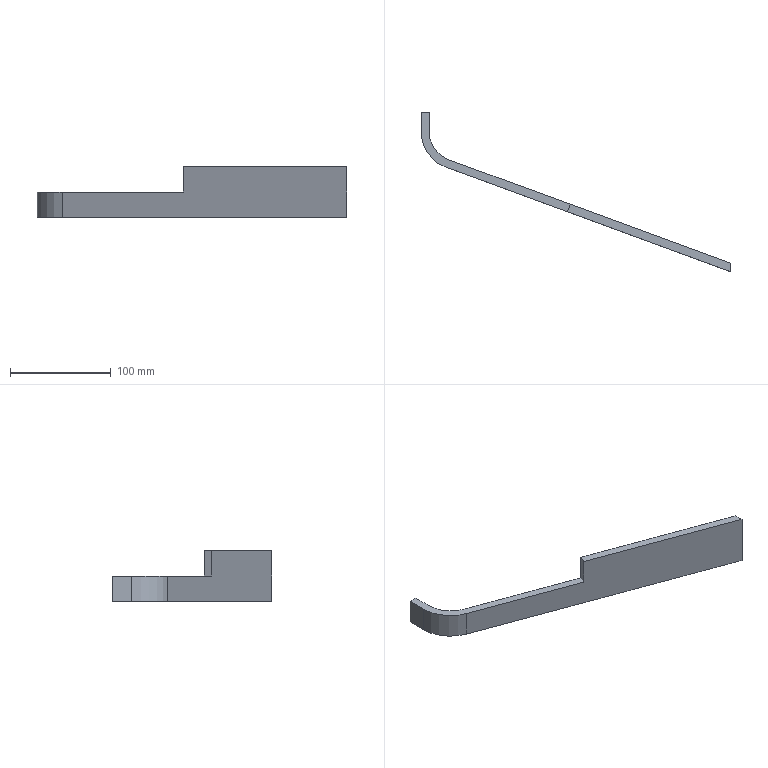Part | SolidWorks | features Extrusion 1, ICE 1 | 1 solid | 12 faces | box 308 x 158.521 x 50 mm | volume 106428 mm3 | plane 10 | cylinder 2 | commonest cylinder face diameters 60 x1 76 x1
STEP:
#1=CARTESIAN_POINT('',(-150.5,75.5,25.));
#2=VERTEX_POINT('',#1);
#3=CARTESIAN_POINT('',(-158.5,75.5,25.));
#4=VERTEX_POINT('',#3);
#5=CARTESIAN_POINT('',(-158.5,75.5,25.));
#6=DIRECTION('',(-1.,0.,0.));
#7=VECTOR('',#6,1000.);
#8=LINE('',#5,#7);
#9=EDGE_CURVE('',#2,#4,#8,.T.);
#10=ORIENTED_EDGE('',*,*,#9,.F.);
#11=CARTESIAN_POINT('',(-150.5,75.5,0.));
#12=VERTEX_POINT('',#11);
#13=CARTESIAN_POINT('',(-150.5,75.5,50.));
#14=DIRECTION('',(0.,0.,-1.));
#15=VECTOR('',#14,1000.);
#16=LINE('',#13,#15);
#17=EDGE_CURVE('',#2,#12,#16,.T.);
#18=ORIENTED_EDGE('',*,*,#17,.T.);
#19=CARTESIAN_POINT('',(-158.5,75.5,0.));
#20=VERTEX_POINT('',#19);
#21=CARTESIAN_POINT('',(-158.5,75.5,0.));
#22=DIRECTION('',(-1.,0.,0.));
#23=VECTOR('',#22,1000.);
#24=LINE('',#21,#23);
#25=EDGE_CURVE('',#12,#20,#24,.T.);
#26=ORIENTED_EDGE('',*,*,#25,.T.);
#27=CARTESIAN_POINT('',(-158.5,75.5,50.));
#28=DIRECTION('',(0.,0.,-1.));
#29=VECTOR('',#28,1000.);
#30=LINE('',#27,#29);
#31=EDGE_CURVE('',#4,#20,#30,.T.);
#32=ORIENTED_EDGE('',*,*,#31,.F.);
#33=EDGE_LOOP('',(#10,#18,#26,#32));
#34=FACE_OUTER_BOUND('',#33,.T.);
#35=CARTESIAN_POINT('',(-158.5,75.5,50.));
#36=DIRECTION('',(0.,-1.,0.));
#37=DIRECTION('',(0.,0.,-1.));
#38=AXIS2_PLACEMENT_3D('',#35,#36,#37);
#39=PLANE('',#38);
#40=ADVANCED_FACE('',(#34),#39,.F.);
#41=CARTESIAN_POINT('',(-158.5,56.453,25.));
#42=VERTEX_POINT('',#41);
#43=CARTESIAN_POINT('',(-158.5,75.5,25.));
#44=DIRECTION('',(0.,-1.,0.));
#45=VECTOR('',#44,1000.);
#46=LINE('',#43,#45);
#47=EDGE_CURVE('',#4,#42,#46,.T.);
#48=ORIENTED_EDGE('',*,*,#47,.F.);
#49=ORIENTED_EDGE('',*,*,#31,.T.);
#50=CARTESIAN_POINT('',(-158.5,56.453,0.));
#51=VERTEX_POINT('',#50);
#52=CARTESIAN_POINT('',(-158.5,75.5,0.));
#53=DIRECTION('',(0.,-1.,0.));
#54=VECTOR('',#53,1000.);
#55=LINE('',#52,#54);
#56=EDGE_CURVE('',#20,#51,#55,.T.);
#57=ORIENTED_EDGE('',*,*,#56,.T.);
#58=CARTESIAN_POINT('',(-158.5,56.453,50.));
#59=DIRECTION('',(0.,0.,-1.));
#60=VECTOR('',#59,1000.);
#61=LINE('',#58,#60);
#62=EDGE_CURVE('',#42,#51,#61,.T.);
#63=ORIENTED_EDGE('',*,*,#62,.F.);
#64=EDGE_LOOP('',(#48,#49,#57,#63));
#65=FACE_OUTER_BOUND('',#64,.T.);
#66=CARTESIAN_POINT('',(-158.5,75.5,50.));
#67=DIRECTION('',(1.,0.,0.));
#68=DIRECTION('',(0.,0.,-1.));
#69=AXIS2_PLACEMENT_3D('',#66,#67,#68);
#70=PLANE('',#69);
#71=ADVANCED_FACE('',(#65),#70,.F.);
#72=CARTESIAN_POINT('',(-133.582,20.776,25.));
#73=VERTEX_POINT('',#72);
#74=CARTESIAN_POINT('',(-120.5,56.453,25.));
#75=DIRECTION('',(0.,0.,1.));
#76=DIRECTION('',(1.,0.,0.));
#77=AXIS2_PLACEMENT_3D('',#74,#75,#76);
#78=CIRCLE('',#77,38.);
#79=EDGE_CURVE('',#42,#73,#78,.T.);
#80=ORIENTED_EDGE('',*,*,#79,.F.);
#81=ORIENTED_EDGE('',*,*,#62,.T.);
#82=CARTESIAN_POINT('',(-133.582,20.776,0.));
#83=VERTEX_POINT('',#82);
#84=CARTESIAN_POINT('',(-120.5,56.453,0.));
#85=DIRECTION('',(0.,0.,1.));
#86=DIRECTION('',(1.,0.,0.));
#87=AXIS2_PLACEMENT_3D('',#84,#85,#86);
#88=CIRCLE('',#87,38.);
#89=EDGE_CURVE('',#51,#83,#88,.T.);
#90=ORIENTED_EDGE('',*,*,#89,.T.);
#91=CARTESIAN_POINT('',(-133.582,20.776,50.));
#92=DIRECTION('',(0.,0.,-1.));
#93=VECTOR('',#92,1000.);
#94=LINE('',#91,#93);
#95=EDGE_CURVE('',#73,#83,#94,.T.);
#96=ORIENTED_EDGE('',*,*,#95,.F.);
#97=EDGE_LOOP('',(#80,#81,#90,#96));
#98=FACE_OUTER_BOUND('',#97,.T.);
#99=CARTESIAN_POINT('',(-120.5,56.453,50.));
#100=DIRECTION('',(0.,0.,-1.));
#101=DIRECTION('',(-1.,0.,0.));
#102=AXIS2_PLACEMENT_3D('',#99,#100,#101);
#103=CYLINDRICAL_SURFACE('',#102,38.);
#104=ADVANCED_FACE('',(#98),#103,.T.);
#105=CARTESIAN_POINT('',(-12.978,-23.446,25.));
#106=VERTEX_POINT('',#105);
#107=CARTESIAN_POINT('',(-9.116,-24.862,25.));
#108=DIRECTION('',(-0.9389,0.3443,0.));
#109=VECTOR('',#108,1000.);
#110=LINE('',#107,#109);
#111=EDGE_CURVE('',#106,#73,#110,.T.);
#112=ORIENTED_EDGE('',*,*,#111,.T.);
#113=ORIENTED_EDGE('',*,*,#95,.T.);
#114=CARTESIAN_POINT('',(149.5,-83.021,0.));
#115=VERTEX_POINT('',#114);
#116=CARTESIAN_POINT('',(146.746,-82.011,0.));
#117=DIRECTION('',(0.9389,-0.3443,0.));
#118=VECTOR('',#117,1000.);
#119=LINE('',#116,#118);
#120=EDGE_CURVE('',#83,#115,#119,.T.);
#121=ORIENTED_EDGE('',*,*,#120,.T.);
#122=CARTESIAN_POINT('',(149.5,-83.021,50.));
#123=VERTEX_POINT('',#122);
#124=CARTESIAN_POINT('',(149.5,-83.021,50.));
#125=DIRECTION('',(0.,0.,-1.));
#126=VECTOR('',#125,1000.);
#127=LINE('',#124,#126);
#128=EDGE_CURVE('',#123,#115,#127,.T.);
#129=ORIENTED_EDGE('',*,*,#128,.F.);
#130=CARTESIAN_POINT('',(-12.978,-23.446,50.));
#131=VERTEX_POINT('',#130);
#132=CARTESIAN_POINT('',(-133.582,20.776,50.));
#133=DIRECTION('',(0.9389,-0.3443,0.));
#134=VECTOR('',#133,1000.);
#135=LINE('',#132,#134);
#136=EDGE_CURVE('',#131,#123,#135,.T.);
#137=ORIENTED_EDGE('',*,*,#136,.F.);
#138=CARTESIAN_POINT('',(-12.978,-23.446,0.));
#139=DIRECTION('',(0.,0.,-1.));
#140=VECTOR('',#139,1000.);
#141=LINE('',#138,#140);
#142=EDGE_CURVE('',#131,#106,#141,.T.);
#143=ORIENTED_EDGE('',*,*,#142,.T.);
#144=EDGE_LOOP('',(#112,#113,#121,#129,#137,#143));
#145=FACE_OUTER_BOUND('',#144,.T.);
#146=CARTESIAN_POINT('',(146.746,-82.011,50.));
#147=DIRECTION('',(0.3443,0.9389,0.));
#148=DIRECTION('',(-0.9389,0.3443,0.));
#149=AXIS2_PLACEMENT_3D('',#146,#147,#148);
#150=PLANE('',#149);
#151=ADVANCED_FACE('',(#145),#150,.F.);
#152=CARTESIAN_POINT('',(-10.224,-15.935,25.));
#153=VERTEX_POINT('',#152);
#154=CARTESIAN_POINT('',(-130.827,28.287,25.));
#155=VERTEX_POINT('',#154);
#156=CARTESIAN_POINT('',(-130.827,28.287,25.));
#157=DIRECTION('',(-0.9389,0.3443,0.));
#158=VECTOR('',#157,1000.);
#159=LINE('',#156,#158);
#160=EDGE_CURVE('',#153,#155,#159,.T.);
#161=ORIENTED_EDGE('',*,*,#160,.F.);
#162=CARTESIAN_POINT('',(-10.224,-15.935,50.));
#163=VERTEX_POINT('',#162);
#164=CARTESIAN_POINT('',(-10.224,-15.935,50.));
#165=DIRECTION('',(0.,0.,-1.));
#166=VECTOR('',#165,1000.);
#167=LINE('',#164,#166);
#168=EDGE_CURVE('',#163,#153,#167,.T.);
#169=ORIENTED_EDGE('',*,*,#168,.F.);
#170=CARTESIAN_POINT('',(149.5,-74.5,50.));
#171=VERTEX_POINT('',#170);
#172=CARTESIAN_POINT('',(-130.827,28.287,50.));
#173=DIRECTION('',(-0.9389,0.3443,0.));
#174=VECTOR('',#173,1000.);
#175=LINE('',#172,#174);
#176=EDGE_CURVE('',#171,#163,#175,.T.);
#177=ORIENTED_EDGE('',*,*,#176,.F.);
#178=CARTESIAN_POINT('',(149.5,-74.5,0.));
#179=VERTEX_POINT('',#178);
#180=CARTESIAN_POINT('',(149.5,-74.5,50.));
#181=DIRECTION('',(0.,0.,-1.));
#182=VECTOR('',#181,1000.);
#183=LINE('',#180,#182);
#184=EDGE_CURVE('',#171,#179,#183,.T.);
#185=ORIENTED_EDGE('',*,*,#184,.T.);
#186=CARTESIAN_POINT('',(-130.827,28.287,0.));
#187=VERTEX_POINT('',#186);
#188=CARTESIAN_POINT('',(-130.827,28.287,0.));
#189=DIRECTION('',(-0.9389,0.3443,0.));
#190=VECTOR('',#189,1000.);
#191=LINE('',#188,#190);
#192=EDGE_CURVE('',#179,#187,#191,.T.);
#193=ORIENTED_EDGE('',*,*,#192,.T.);
#194=CARTESIAN_POINT('',(-130.827,28.287,50.));
#195=DIRECTION('',(0.,0.,-1.));
#196=VECTOR('',#195,1000.);
#197=LINE('',#194,#196);
#198=EDGE_CURVE('',#155,#187,#197,.T.);
#199=ORIENTED_EDGE('',*,*,#198,.F.);
#200=EDGE_LOOP('',(#161,#169,#177,#185,#193,#199));
#201=FACE_OUTER_BOUND('',#200,.T.);
#202=CARTESIAN_POINT('',(-130.827,28.287,50.));
#203=DIRECTION('',(-0.3443,-0.9389,0.));
#204=DIRECTION('',(0.9389,-0.3443,0.));
#205=AXIS2_PLACEMENT_3D('',#202,#203,#204);
#206=PLANE('',#205);
#207=ADVANCED_FACE('',(#201),#206,.F.);
#208=CARTESIAN_POINT('',(-150.5,56.453,25.));
#209=VERTEX_POINT('',#208);
#210=CARTESIAN_POINT('',(-120.5,56.453,25.));
#211=DIRECTION('',(0.,0.,-1.));
#212=DIRECTION('',(1.,0.,0.));
#213=AXIS2_PLACEMENT_3D('',#210,#211,#212);
#214=CIRCLE('',#213,30.);
#215=EDGE_CURVE('',#155,#209,#214,.T.);
#216=ORIENTED_EDGE('',*,*,#215,.F.);
#217=ORIENTED_EDGE('',*,*,#198,.T.);
#218=CARTESIAN_POINT('',(-150.5,56.453,0.));
#219=VERTEX_POINT('',#218);
#220=CARTESIAN_POINT('',(-120.5,56.453,0.));
#221=DIRECTION('',(0.,0.,-1.));
#222=DIRECTION('',(1.,0.,0.));
#223=AXIS2_PLACEMENT_3D('',#220,#221,#222);
#224=CIRCLE('',#223,30.);
#225=EDGE_CURVE('',#187,#219,#224,.T.);
#226=ORIENTED_EDGE('',*,*,#225,.T.);
#227=CARTESIAN_POINT('',(-150.5,56.453,50.));
#228=DIRECTION('',(0.,0.,-1.));
#229=VECTOR('',#228,1000.);
#230=LINE('',#227,#229);
#231=EDGE_CURVE('',#209,#219,#230,.T.);
#232=ORIENTED_EDGE('',*,*,#231,.F.);
#233=EDGE_LOOP('',(#216,#217,#226,#232));
#234=FACE_OUTER_BOUND('',#233,.T.);
#235=CARTESIAN_POINT('',(-120.5,56.453,50.));
#236=DIRECTION('',(0.,0.,-1.));
#237=DIRECTION('',(-1.,0.,0.));
#238=AXIS2_PLACEMENT_3D('',#235,#236,#237);
#239=CYLINDRICAL_SURFACE('',#238,30.);
#240=ADVANCED_FACE('',(#234),#239,.F.);
#241=CARTESIAN_POINT('',(-150.5,75.5,25.));
#242=DIRECTION('',(0.,1.,0.));
#243=VECTOR('',#242,1000.);
#244=LINE('',#241,#243);
#245=EDGE_CURVE('',#209,#2,#244,.T.);
#246=ORIENTED_EDGE('',*,*,#245,.F.);
#247=ORIENTED_EDGE('',*,*,#231,.T.);
#248=CARTESIAN_POINT('',(-150.5,75.5,0.));
#249=DIRECTION('',(0.,1.,0.));
#250=VECTOR('',#249,1000.);
#251=LINE('',#248,#250);
#252=EDGE_CURVE('',#219,#12,#251,.T.);
#253=ORIENTED_EDGE('',*,*,#252,.T.);
#254=ORIENTED_EDGE('',*,*,#17,.F.);
#255=EDGE_LOOP('',(#246,#247,#253,#254));
#256=FACE_OUTER_BOUND('',#255,.T.);
#257=CARTESIAN_POINT('',(-150.5,75.5,50.));
#258=DIRECTION('',(-1.,0.,0.));
#259=DIRECTION('',(0.,0.,1.));
#260=AXIS2_PLACEMENT_3D('',#257,#258,#259);
#261=PLANE('',#260);
#262=ADVANCED_FACE('',(#256),#261,.F.);
#263=ORIENTED_EDGE('',*,*,#176,.T.);
#264=CARTESIAN_POINT('',(0.1041,12.231,50.));
#265=DIRECTION('',(-0.3443,-0.9389,0.));
#266=VECTOR('',#265,1000.);
#267=LINE('',#264,#266);
#268=EDGE_CURVE('',#163,#131,#267,.T.);
#269=ORIENTED_EDGE('',*,*,#268,.T.);
#270=ORIENTED_EDGE('',*,*,#136,.T.);
#271=CARTESIAN_POINT('',(149.5,-74.5,50.));
#272=DIRECTION('',(0.,1.,0.));
#273=VECTOR('',#272,1000.);
#274=LINE('',#271,#273);
#275=EDGE_CURVE('',#123,#171,#274,.T.);
#276=ORIENTED_EDGE('',*,*,#275,.T.);
#277=EDGE_LOOP('',(#263,#269,#270,#276));
#278=FACE_OUTER_BOUND('',#277,.T.);
#279=CARTESIAN_POINT('',(-120.5,56.453,50.));
#280=DIRECTION('',(0.,0.,1.));
#281=DIRECTION('',(1.,0.,0.));
#282=AXIS2_PLACEMENT_3D('',#279,#280,#281);
#283=PLANE('',#282);
#284=ADVANCED_FACE('',(#278),#283,.T.);
#285=CARTESIAN_POINT('',(149.5,-74.5,0.));
#286=DIRECTION('',(0.,1.,0.));
#287=VECTOR('',#286,1000.);
#288=LINE('',#285,#287);
#289=EDGE_CURVE('',#115,#179,#288,.T.);
#290=ORIENTED_EDGE('',*,*,#289,.T.);
#291=ORIENTED_EDGE('',*,*,#184,.F.);
#292=ORIENTED_EDGE('',*,*,#275,.F.);
#293=ORIENTED_EDGE('',*,*,#128,.T.);
#294=EDGE_LOOP('',(#290,#291,#292,#293));
#295=FACE_OUTER_BOUND('',#294,.T.);
#296=CARTESIAN_POINT('',(149.5,-74.5,50.));
#297=DIRECTION('',(-1.,0.,0.));
#298=DIRECTION('',(0.,0.,1.));
#299=AXIS2_PLACEMENT_3D('',#296,#297,#298);
#300=PLANE('',#299);
#301=ADVANCED_FACE('',(#295),#300,.F.);
#302=ORIENTED_EDGE('',*,*,#25,.F.);
#303=ORIENTED_EDGE('',*,*,#252,.F.);
#304=ORIENTED_EDGE('',*,*,#225,.F.);
#305=ORIENTED_EDGE('',*,*,#192,.F.);
#306=ORIENTED_EDGE('',*,*,#289,.F.);
#307=ORIENTED_EDGE('',*,*,#120,.F.);
#308=ORIENTED_EDGE('',*,*,#89,.F.);
#309=ORIENTED_EDGE('',*,*,#56,.F.);
#310=EDGE_LOOP('',(#302,#303,#304,#305,#306,#307,#308,#309));
#311=FACE_OUTER_BOUND('',#310,.T.);
#312=CARTESIAN_POINT('',(-120.5,56.453,0.));
#313=DIRECTION('',(0.,0.,1.));
#314=DIRECTION('',(1.,0.,0.));
#315=AXIS2_PLACEMENT_3D('',#312,#313,#314);
#316=PLANE('',#315);
#317=ADVANCED_FACE('',(#311),#316,.F.);
#318=ORIENTED_EDGE('',*,*,#79,.T.);
#319=ORIENTED_EDGE('',*,*,#111,.F.);
#320=CARTESIAN_POINT('',(3.891,22.559,25.));
#321=DIRECTION('',(-0.3443,-0.9389,0.));
#322=VECTOR('',#321,1000.);
#323=LINE('',#320,#322);
#324=EDGE_CURVE('',#153,#106,#323,.T.);
#325=ORIENTED_EDGE('',*,*,#324,.F.);
#326=ORIENTED_EDGE('',*,*,#160,.T.);
#327=ORIENTED_EDGE('',*,*,#215,.T.);
#328=ORIENTED_EDGE('',*,*,#245,.T.);
#329=ORIENTED_EDGE('',*,*,#9,.T.);
#330=ORIENTED_EDGE('',*,*,#47,.T.);
#331=EDGE_LOOP('',(#318,#319,#325,#326,#327,#328,#329,#330));
#332=FACE_OUTER_BOUND('',#331,.T.);
#333=CARTESIAN_POINT('',(7.753,21.143,25.));
#334=DIRECTION('',(0.,0.,1.));
#335=DIRECTION('',(1.,0.,0.));
#336=AXIS2_PLACEMENT_3D('',#333,#334,#335);
#337=PLANE('',#336);
#338=ADVANCED_FACE('',(#332),#337,.T.);
#339=ORIENTED_EDGE('',*,*,#168,.T.);
#340=ORIENTED_EDGE('',*,*,#324,.T.);
#341=ORIENTED_EDGE('',*,*,#142,.F.);
#342=ORIENTED_EDGE('',*,*,#268,.F.);
#343=EDGE_LOOP('',(#339,#340,#341,#342));
#344=FACE_OUTER_BOUND('',#343,.T.);
#345=CARTESIAN_POINT('',(3.891,22.559,0.));
#346=DIRECTION('',(-0.9389,0.3443,0.));
#347=DIRECTION('',(-0.3443,-0.9389,0.));
#348=AXIS2_PLACEMENT_3D('',#345,#346,#347);
#349=PLANE('',#348);
#350=ADVANCED_FACE('',(#344),#349,.T.);
#351=CLOSED_SHELL('',(#40,#71,#104,#151,#207,#240,#262,#284,#301,#317,#338,#350));
#352=MANIFOLD_SOLID_BREP('',#351);
#353=CARTESIAN_POINT('',(0.,0.,0.));
#354=DIRECTION('',(0.,0.,1.));
#355=DIRECTION('',(1.,0.,0.));
#356=AXIS2_PLACEMENT_3D('',#353,#354,#355);
#357=(LENGTH_UNIT()NAMED_UNIT(*)SI_UNIT(.MILLI.,.METRE.));
#358=UNCERTAINTY_MEASURE_WITH_UNIT(LENGTH_MEASURE(0.00001),#357,'','');
#359=(NAMED_UNIT(*)PLANE_ANGLE_UNIT()SI_UNIT($,.RADIAN.));
#360=(NAMED_UNIT(*)SI_UNIT($,.STERADIAN.)SOLID_ANGLE_UNIT());
#361=(GEOMETRIC_REPRESENTATION_CONTEXT(3)GLOBAL_UNCERTAINTY_ASSIGNED_CONTEXT((#358))GLOBAL_UNIT_ASSIGNED_CONTEXT((#357,#359,#360))REPRESENTATION_CONTEXT('',''));
#362=ADVANCED_BREP_SHAPE_REPRESENTATION('',(#352,#356),#361);